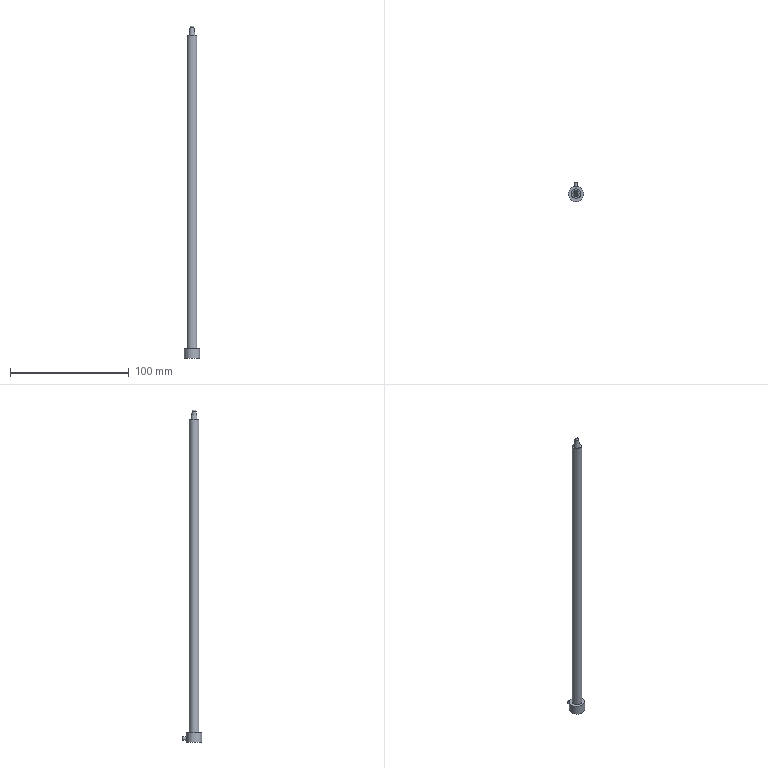Part | STEP file | E108-15-310 | 1 solid | 11 faces | box 13 x 16.5 x 280 mm | volume 14461 mm3 | plane 5 | cylinder 3 | cone 2 | spline 1 | commonest cylinder face diameters 3 x1 8 x1 13 x1
STEP:
#1=CARTESIAN_POINT('',(0.,0.,0.));
#2=DIRECTION('',(0.,0.,1.));
#3=DIRECTION('',(1.,0.,0.));
#4=AXIS2_PLACEMENT_3D('',#1,#2,#3);
#5=CARTESIAN_POINT('',(-4.,0.,272.));
#6=VERTEX_POINT('',#5);
#7=CARTESIAN_POINT('',(4.,0.,272.));
#8=VERTEX_POINT('',#7);
#9=CARTESIAN_POINT('',(0.,0.,272.));
#10=DIRECTION('',(0.,0.,1.));
#11=DIRECTION('',(1.,0.,0.));
#12=AXIS2_PLACEMENT_3D('',#9,#10,#11);
#13=CIRCLE('',#12,4.);
#14=CARTESIAN_POINT('',(0.,0.,100.));
#15=DIRECTION('',(0.,0.,-1.));
#16=DIRECTION('',(-1.,0.,0.));
#17=AXIS2_PLACEMENT_3D('',#14,#15,#16);
#18=CYLINDRICAL_SURFACE('',#17,4.);
#19=CARTESIAN_POINT('',(9.425,-172.));
#20=DIRECTION('',(-1.,0.));
#21=VECTOR('',#20,1.);
#22=LINE('',#19,#21);
#23=(GEOMETRIC_REPRESENTATION_CONTEXT(2)PARAMETRIC_REPRESENTATION_CONTEXT()REPRESENTATION_CONTEXT('',''));
#24=DEFINITIONAL_REPRESENTATION('',(#22),#23);
#25=PCURVE('',#18,#24);
#26=CARTESIAN_POINT('',(0.,0.,272.));
#27=DIRECTION('',(0.,0.,1.));
#28=DIRECTION('',(1.,0.,0.));
#29=AXIS2_PLACEMENT_3D('',#26,#27,#28);
#30=PLANE('',#29);
#31=CARTESIAN_POINT('',(0.,0.));
#32=DIRECTION('',(1.,0.));
#33=AXIS2_PLACEMENT_2D('',#31,#32);
#34=CIRCLE('',#33,4.);
#35=(GEOMETRIC_REPRESENTATION_CONTEXT(2)PARAMETRIC_REPRESENTATION_CONTEXT()REPRESENTATION_CONTEXT('',''));
#36=DEFINITIONAL_REPRESENTATION('',(#34),#35);
#37=PCURVE('',#30,#36);
#38=SURFACE_CURVE('',#13,(#25,#37),.PCURVE_S1.);
#39=EDGE_CURVE('',#6,#8,#38,.T.);
#40=ORIENTED_EDGE('',*,*,#39,.F.);
#41=CARTESIAN_POINT('',(-4.,0.,8.));
#42=VERTEX_POINT('',#41);
#43=CARTESIAN_POINT('',(-4.,0.,272.));
#44=CARTESIAN_POINT('',(-4.,0.,8.));
#45=B_SPLINE_CURVE_WITH_KNOTS('',1,(#43,#44),.UNSPECIFIED.,.F.,.F.,(2,2),(-172.,92.),.PIECEWISE_BEZIER_KNOTS.);
#46=CARTESIAN_POINT('',(6.283,0.));
#47=DIRECTION('',(0.,1.));
#48=VECTOR('',#47,1.);
#49=LINE('',#46,#48);
#50=(GEOMETRIC_REPRESENTATION_CONTEXT(2)PARAMETRIC_REPRESENTATION_CONTEXT()REPRESENTATION_CONTEXT('',''));
#51=DEFINITIONAL_REPRESENTATION('',(#49),#50);
#52=PCURVE('',#18,#51);
#53=CARTESIAN_POINT('',(0.,0.));
#54=DIRECTION('',(0.,1.));
#55=VECTOR('',#54,1.);
#56=LINE('',#53,#55);
#57=(GEOMETRIC_REPRESENTATION_CONTEXT(2)PARAMETRIC_REPRESENTATION_CONTEXT()REPRESENTATION_CONTEXT('',''));
#58=DEFINITIONAL_REPRESENTATION('',(#56),#57);
#59=PCURVE('',#18,#58);
#60=SEAM_CURVE('',#45,(#52,#59),.PCURVE_S1.);
#61=EDGE_CURVE('',#6,#42,#60,.T.);
#62=ORIENTED_EDGE('',*,*,#61,.T.);
#63=CARTESIAN_POINT('',(0.,0.,8.));
#64=DIRECTION('',(0.,0.,1.));
#65=DIRECTION('',(-1.,0.,0.));
#66=AXIS2_PLACEMENT_3D('',#63,#64,#65);
#67=CIRCLE('',#66,4.);
#68=CARTESIAN_POINT('',(6.283,92.));
#69=DIRECTION('',(-1.,0.));
#70=VECTOR('',#69,1.);
#71=LINE('',#68,#70);
#72=(GEOMETRIC_REPRESENTATION_CONTEXT(2)PARAMETRIC_REPRESENTATION_CONTEXT()REPRESENTATION_CONTEXT('',''));
#73=DEFINITIONAL_REPRESENTATION('',(#71),#72);
#74=PCURVE('',#18,#73);
#75=CARTESIAN_POINT('',(0.,0.,8.));
#76=DIRECTION('',(0.,0.,-1.));
#77=DIRECTION('',(1.,0.,0.));
#78=AXIS2_PLACEMENT_3D('',#75,#76,#77);
#79=PLANE('',#78);
#80=CARTESIAN_POINT('',(-4.,0.));
#81=CARTESIAN_POINT('',(-4.,6.928));
#82=CARTESIAN_POINT('',(2.,3.464));
#83=CARTESIAN_POINT('',(8.,0.));
#84=CARTESIAN_POINT('',(2.,-3.464));
#85=CARTESIAN_POINT('',(-4.,-6.928));
#86=CARTESIAN_POINT('',(-4.,0.));
#87=(BOUNDED_CURVE()B_SPLINE_CURVE(2,(#80,#81,#82,#83,#84,#85,#86),.UNSPECIFIED.,.T.,.F.)B_SPLINE_CURVE_WITH_KNOTS((1,2,2,2,2,1),(-2.094,0.,2.094,4.189,6.283,8.378),.UNSPECIFIED.)CURVE()GEOMETRIC_REPRESENTATION_ITEM()RATIONAL_B_SPLINE_CURVE((1.,0.5,1.,0.5,1.,0.5,1.))REPRESENTATION_ITEM(''));
#88=(GEOMETRIC_REPRESENTATION_CONTEXT(2)PARAMETRIC_REPRESENTATION_CONTEXT()REPRESENTATION_CONTEXT('',''));
#89=DEFINITIONAL_REPRESENTATION('',(#87),#88);
#90=PCURVE('',#79,#89);
#91=SURFACE_CURVE('',#67,(#74,#90),.PCURVE_S1.);
#92=EDGE_CURVE('',#42,#42,#91,.T.);
#93=ORIENTED_EDGE('',*,*,#92,.T.);
#94=ORIENTED_EDGE('',*,*,#61,.F.);
#95=CARTESIAN_POINT('',(0.,0.,272.));
#96=DIRECTION('',(0.,0.,1.));
#97=DIRECTION('',(1.,0.,0.));
#98=AXIS2_PLACEMENT_3D('',#95,#96,#97);
#99=CIRCLE('',#98,4.);
#100=CARTESIAN_POINT('',(3.142,-172.));
#101=DIRECTION('',(-1.,0.));
#102=VECTOR('',#101,1.);
#103=LINE('',#100,#102);
#104=(GEOMETRIC_REPRESENTATION_CONTEXT(2)PARAMETRIC_REPRESENTATION_CONTEXT()REPRESENTATION_CONTEXT('',''));
#105=DEFINITIONAL_REPRESENTATION('',(#103),#104);
#106=PCURVE('',#18,#105);
#107=CARTESIAN_POINT('',(0.,0.));
#108=DIRECTION('',(1.,0.));
#109=AXIS2_PLACEMENT_2D('',#107,#108);
#110=CIRCLE('',#109,4.);
#111=(GEOMETRIC_REPRESENTATION_CONTEXT(2)PARAMETRIC_REPRESENTATION_CONTEXT()REPRESENTATION_CONTEXT('',''));
#112=DEFINITIONAL_REPRESENTATION('',(#110),#111);
#113=PCURVE('',#30,#112);
#114=SURFACE_CURVE('',#99,(#106,#113),.PCURVE_S1.);
#115=EDGE_CURVE('',#8,#6,#114,.T.);
#116=ORIENTED_EDGE('',*,*,#115,.F.);
#117=EDGE_LOOP('',(#40,#62,#93,#94,#116));
#118=FACE_BOUND('',#117,.T.);
#119=ADVANCED_FACE('',(#118),#18,.T.);
#120=CARTESIAN_POINT('',(2.553,0.,272.));
#121=VERTEX_POINT('',#120);
#122=CARTESIAN_POINT('',(0.,0.,272.));
#123=DIRECTION('',(0.,0.,1.));
#124=DIRECTION('',(1.,0.,0.));
#125=AXIS2_PLACEMENT_3D('',#122,#123,#124);
#126=CIRCLE('',#125,2.553);
#127=CARTESIAN_POINT('',(0.,0.));
#128=DIRECTION('',(1.,0.));
#129=AXIS2_PLACEMENT_2D('',#127,#128);
#130=CIRCLE('',#129,2.553);
#131=(GEOMETRIC_REPRESENTATION_CONTEXT(2)PARAMETRIC_REPRESENTATION_CONTEXT()REPRESENTATION_CONTEXT('',''));
#132=DEFINITIONAL_REPRESENTATION('',(#130),#131);
#133=PCURVE('',#30,#132);
#134=CARTESIAN_POINT('',(0.,0.,280.));
#135=DIRECTION('',(0.,0.,-1.));
#136=DIRECTION('',(-1.,0.,0.));
#137=AXIS2_PLACEMENT_3D('',#134,#135,#136);
#138=CONICAL_SURFACE('',#137,1.5,0.1309);
#139=CARTESIAN_POINT('',(9.425,8.));
#140=DIRECTION('',(-1.,0.));
#141=VECTOR('',#140,1.);
#142=LINE('',#139,#141);
#143=(GEOMETRIC_REPRESENTATION_CONTEXT(2)PARAMETRIC_REPRESENTATION_CONTEXT()REPRESENTATION_CONTEXT('',''));
#144=DEFINITIONAL_REPRESENTATION('',(#142),#143);
#145=PCURVE('',#138,#144);
#146=SURFACE_CURVE('',#126,(#133,#145),.PCURVE_S1.);
#147=EDGE_CURVE('',#121,#121,#146,.T.);
#148=ORIENTED_EDGE('',*,*,#147,.F.);
#149=EDGE_LOOP('',(#148));
#150=FACE_BOUND('',#149,.T.);
#151=ORIENTED_EDGE('',*,*,#115,.T.);
#152=ORIENTED_EDGE('',*,*,#39,.T.);
#153=EDGE_LOOP('',(#151,#152));
#154=FACE_BOUND('',#153,.T.);
#155=ADVANCED_FACE('',(#150,#154),#30,.T.);
#156=CARTESIAN_POINT('',(6.5,0.,0.));
#157=VERTEX_POINT('',#156);
#158=CARTESIAN_POINT('',(-6.5,0.,0.));
#159=VERTEX_POINT('',#158);
#160=CARTESIAN_POINT('',(0.,0.,0.));
#161=DIRECTION('',(0.,0.,-1.));
#162=DIRECTION('',(-1.,0.,0.));
#163=AXIS2_PLACEMENT_3D('',#160,#161,#162);
#164=CIRCLE('',#163,6.5);
#165=CARTESIAN_POINT('',(0.,0.,8.));
#166=DIRECTION('',(0.,0.,-1.));
#167=DIRECTION('',(1.,0.,0.));
#168=AXIS2_PLACEMENT_3D('',#165,#166,#167);
#169=CYLINDRICAL_SURFACE('',#168,6.5);
#170=CARTESIAN_POINT('',(-3.142,8.));
#171=DIRECTION('',(1.,0.));
#172=VECTOR('',#171,1.);
#173=LINE('',#170,#172);
#174=(GEOMETRIC_REPRESENTATION_CONTEXT(2)PARAMETRIC_REPRESENTATION_CONTEXT()REPRESENTATION_CONTEXT('',''));
#175=DEFINITIONAL_REPRESENTATION('',(#173),#174);
#176=PCURVE('',#169,#175);
#177=CARTESIAN_POINT('',(240.,-1000.,0.));
#178=DIRECTION('',(0.,0.,1.));
#179=DIRECTION('',(-1.,0.,0.));
#180=AXIS2_PLACEMENT_3D('',#177,#178,#179);
#181=PLANE('',#180);
#182=CARTESIAN_POINT('',(246.5,-1000.));
#183=CARTESIAN_POINT('',(246.5,-1011.258));
#184=CARTESIAN_POINT('',(236.75,-1005.629));
#185=CARTESIAN_POINT('',(227.,-1000.));
#186=CARTESIAN_POINT('',(236.75,-994.371));
#187=CARTESIAN_POINT('',(246.5,-988.742));
#188=CARTESIAN_POINT('',(246.5,-1000.));
#189=(BOUNDED_CURVE()B_SPLINE_CURVE(2,(#182,#183,#184,#185,#186,#187,#188),.UNSPECIFIED.,.T.,.F.)B_SPLINE_CURVE_WITH_KNOTS((1,2,2,2,2,1),(-2.094,0.,2.094,4.189,6.283,8.378),.UNSPECIFIED.)CURVE()GEOMETRIC_REPRESENTATION_ITEM()RATIONAL_B_SPLINE_CURVE((1.,0.5,1.,0.5,1.,0.5,1.))REPRESENTATION_ITEM(''));
#190=(GEOMETRIC_REPRESENTATION_CONTEXT(2)PARAMETRIC_REPRESENTATION_CONTEXT()REPRESENTATION_CONTEXT('',''));
#191=DEFINITIONAL_REPRESENTATION('',(#189),#190);
#192=PCURVE('',#181,#191);
#193=SURFACE_CURVE('',#164,(#176,#192),.PCURVE_S1.);
#194=EDGE_CURVE('',#157,#159,#193,.T.);
#195=ORIENTED_EDGE('',*,*,#194,.F.);
#196=CARTESIAN_POINT('',(6.5,0.,8.));
#197=VERTEX_POINT('',#196);
#198=CARTESIAN_POINT('',(6.5,0.,8.));
#199=CARTESIAN_POINT('',(6.5,0.,0.));
#200=B_SPLINE_CURVE_WITH_KNOTS('',1,(#198,#199),.UNSPECIFIED.,.F.,.F.,(2,2),(0.,8.),.PIECEWISE_BEZIER_KNOTS.);
#201=CARTESIAN_POINT('',(0.,0.));
#202=DIRECTION('',(0.,1.));
#203=VECTOR('',#202,1.);
#204=LINE('',#201,#203);
#205=(GEOMETRIC_REPRESENTATION_CONTEXT(2)PARAMETRIC_REPRESENTATION_CONTEXT()REPRESENTATION_CONTEXT('',''));
#206=DEFINITIONAL_REPRESENTATION('',(#204),#205);
#207=PCURVE('',#169,#206);
#208=CARTESIAN_POINT('',(6.283,0.));
#209=DIRECTION('',(0.,1.));
#210=VECTOR('',#209,1.);
#211=LINE('',#208,#210);
#212=(GEOMETRIC_REPRESENTATION_CONTEXT(2)PARAMETRIC_REPRESENTATION_CONTEXT()REPRESENTATION_CONTEXT('',''));
#213=DEFINITIONAL_REPRESENTATION('',(#211),#212);
#214=PCURVE('',#169,#213);
#215=SEAM_CURVE('',#200,(#207,#214),.PCURVE_S1.);
#216=EDGE_CURVE('',#197,#157,#215,.T.);
#217=ORIENTED_EDGE('',*,*,#216,.F.);
#218=CARTESIAN_POINT('',(0.,0.,8.));
#219=DIRECTION('',(0.,0.,-1.));
#220=DIRECTION('',(1.,0.,0.));
#221=AXIS2_PLACEMENT_3D('',#218,#219,#220);
#222=CIRCLE('',#221,6.5);
#223=CARTESIAN_POINT('',(0.,0.));
#224=DIRECTION('',(1.,0.));
#225=VECTOR('',#224,1.);
#226=LINE('',#223,#225);
#227=(GEOMETRIC_REPRESENTATION_CONTEXT(2)PARAMETRIC_REPRESENTATION_CONTEXT()REPRESENTATION_CONTEXT('',''));
#228=DEFINITIONAL_REPRESENTATION('',(#226),#227);
#229=PCURVE('',#169,#228);
#230=CARTESIAN_POINT('',(0.,0.));
#231=DIRECTION('',(1.,0.));
#232=AXIS2_PLACEMENT_2D('',#230,#231);
#233=CIRCLE('',#232,6.5);
#234=(GEOMETRIC_REPRESENTATION_CONTEXT(2)PARAMETRIC_REPRESENTATION_CONTEXT()REPRESENTATION_CONTEXT('',''));
#235=DEFINITIONAL_REPRESENTATION('',(#233),#234);
#236=PCURVE('',#79,#235);
#237=SURFACE_CURVE('',#222,(#229,#236),.PCURVE_S1.);
#238=EDGE_CURVE('',#197,#197,#237,.T.);
#239=ORIENTED_EDGE('',*,*,#238,.T.);
#240=ORIENTED_EDGE('',*,*,#216,.T.);
#241=CARTESIAN_POINT('',(0.,0.,0.));
#242=DIRECTION('',(0.,0.,-1.));
#243=DIRECTION('',(-1.,0.,0.));
#244=AXIS2_PLACEMENT_3D('',#241,#242,#243);
#245=CIRCLE('',#244,6.5);
#246=CARTESIAN_POINT('',(3.142,8.));
#247=DIRECTION('',(1.,0.));
#248=VECTOR('',#247,1.);
#249=LINE('',#246,#248);
#250=(GEOMETRIC_REPRESENTATION_CONTEXT(2)PARAMETRIC_REPRESENTATION_CONTEXT()REPRESENTATION_CONTEXT('',''));
#251=DEFINITIONAL_REPRESENTATION('',(#249),#250);
#252=PCURVE('',#169,#251);
#253=CARTESIAN_POINT('',(246.5,-1000.));
#254=CARTESIAN_POINT('',(246.5,-1011.258));
#255=CARTESIAN_POINT('',(236.75,-1005.629));
#256=CARTESIAN_POINT('',(227.,-1000.));
#257=CARTESIAN_POINT('',(236.75,-994.371));
#258=CARTESIAN_POINT('',(246.5,-988.742));
#259=CARTESIAN_POINT('',(246.5,-1000.));
#260=(BOUNDED_CURVE()B_SPLINE_CURVE(2,(#253,#254,#255,#256,#257,#258,#259),.UNSPECIFIED.,.T.,.F.)B_SPLINE_CURVE_WITH_KNOTS((1,2,2,2,2,1),(-2.094,0.,2.094,4.189,6.283,8.378),.UNSPECIFIED.)CURVE()GEOMETRIC_REPRESENTATION_ITEM()RATIONAL_B_SPLINE_CURVE((1.,0.5,1.,0.5,1.,0.5,1.))REPRESENTATION_ITEM(''));
#261=(GEOMETRIC_REPRESENTATION_CONTEXT(2)PARAMETRIC_REPRESENTATION_CONTEXT()REPRESENTATION_CONTEXT('',''));
#262=DEFINITIONAL_REPRESENTATION('',(#260),#261);
#263=PCURVE('',#181,#262);
#264=SURFACE_CURVE('',#245,(#252,#263),.PCURVE_S1.);
#265=EDGE_CURVE('',#159,#157,#264,.T.);
#266=ORIENTED_EDGE('',*,*,#265,.F.);
#267=EDGE_LOOP('',(#195,#217,#239,#240,#266));
#268=FACE_BOUND('',#267,.T.);
#269=CARTESIAN_POINT('',(0.,6.5,1.5));
#270=VERTEX_POINT('',#269);
#271=CARTESIAN_POINT('',(0.,6.5,1.5));
#272=CARTESIAN_POINT('',(0.1654,6.5,1.5));
#273=CARTESIAN_POINT('',(0.3332,6.493,1.528));
#274=CARTESIAN_POINT('',(0.4892,6.482,1.582));
#275=CARTESIAN_POINT('',(0.6451,6.47,1.636));
#276=CARTESIAN_POINT('',(0.7936,6.453,1.717));
#277=CARTESIAN_POINT('',(0.9231,6.434,1.818));
#278=CARTESIAN_POINT('',(1.055,6.415,1.92));
#279=CARTESIAN_POINT('',(1.17,6.394,2.047));
#280=CARTESIAN_POINT('',(1.261,6.377,2.187));
#281=CARTESIAN_POINT('',(1.352,6.358,2.329));
#282=CARTESIAN_POINT('',(1.421,6.343,2.49));
#283=CARTESIAN_POINT('',(1.46,6.334,2.655));
#284=CARTESIAN_POINT('',(1.498,6.325,2.817));
#285=CARTESIAN_POINT('',(1.509,6.322,2.989));
#286=CARTESIAN_POINT('',(1.492,6.326,3.155));
#287=CARTESIAN_POINT('',(1.475,6.33,3.318));
#288=CARTESIAN_POINT('',(1.431,6.341,3.48));
#289=CARTESIAN_POINT('',(1.362,6.356,3.628));
#290=CARTESIAN_POINT('',(1.293,6.37,3.777));
#291=CARTESIAN_POINT('',(1.199,6.39,3.917));
#292=CARTESIAN_POINT('',(1.085,6.409,4.035));
#293=CARTESIAN_POINT('',(0.9695,6.428,4.157));
#294=CARTESIAN_POINT('',(0.8309,6.448,4.26));
#295=CARTESIAN_POINT('',(0.6809,6.464,4.337));
#296=CARTESIAN_POINT('',(0.5305,6.48,4.413));
#297=CARTESIAN_POINT('',(0.3642,6.492,4.465));
#298=CARTESIAN_POINT('',(0.1962,6.497,4.487));
#299=CARTESIAN_POINT('',(0.03191,6.502,4.509));
#300=CARTESIAN_POINT('',(-0.1386,6.501,4.503));
#301=CARTESIAN_POINT('',(-0.3008,6.493,4.47));
#302=CARTESIAN_POINT('',(-0.4611,6.486,4.437));
#303=CARTESIAN_POINT('',(-0.6177,6.472,4.377));
#304=CARTESIAN_POINT('',(-0.7583,6.456,4.294));
#305=CARTESIAN_POINT('',(-0.9011,6.439,4.211));
#306=CARTESIAN_POINT('',(-1.031,6.419,4.102));
#307=CARTESIAN_POINT('',(-1.139,6.399,3.976));
#308=CARTESIAN_POINT('',(-1.249,6.38,3.848));
#309=CARTESIAN_POINT('',(-1.338,6.361,3.699));
#310=CARTESIAN_POINT('',(-1.399,6.348,3.541));
#311=CARTESIAN_POINT('',(-1.46,6.334,3.384));
#312=CARTESIAN_POINT('',(-1.494,6.326,3.214));
#313=CARTESIAN_POINT('',(-1.499,6.325,3.046));
#314=CARTESIAN_POINT('',(-1.504,6.324,2.881));
#315=CARTESIAN_POINT('',(-1.482,6.329,2.714));
#316=CARTESIAN_POINT('',(-1.433,6.34,2.557));
#317=CARTESIAN_POINT('',(-1.385,6.351,2.4));
#318=CARTESIAN_POINT('',(-1.309,6.367,2.25));
#319=CARTESIAN_POINT('',(-1.214,6.386,2.119));
#320=CARTESIAN_POINT('',(-1.116,6.404,1.984));
#321=CARTESIAN_POINT('',(-0.9937,6.425,1.864));
#322=CARTESIAN_POINT('',(-0.8569,6.443,1.769));
#323=CARTESIAN_POINT('',(-0.7182,6.462,1.672));
#324=CARTESIAN_POINT('',(-0.5604,6.478,1.598));
#325=CARTESIAN_POINT('',(-0.3967,6.488,1.553));
#326=CARTESIAN_POINT('',(-0.2682,6.496,1.518));
#327=CARTESIAN_POINT('',(-0.1335,6.5,1.5));
#328=CARTESIAN_POINT('',(0.,6.5,1.5));
#329=B_SPLINE_CURVE_WITH_KNOTS('',3,(#271,#272,#273,#274,#275,#276,#277,#278,#279,#280,#281,#282,#283,#284,#285,#286,#287,#288,#289,#290,#291,#292,#293,#294,#295,#296,#297,#298,#299,#300,#301,#302,#303,#304,#305,#306,#307,#308,#309,#310,#311,#312,#313,#314,#315,#316,#317,#318,#319,#320,#321,#322,#323,#324,#325,#326,#327,#328),.UNSPECIFIED.,.T.,.F.,(1,3,3,3,3,3,3,3,3,3,3,3,3,3,3,3,3,3,3,3,3,1),(-0.04234,0.,0.05275,0.1054,0.159,0.2132,0.2665,0.3187,0.3713,0.4252,0.4793,0.5321,0.5843,0.6373,0.6915,0.7453,0.7978,0.85,0.9034,0.9577,1.,1.053),.UNSPECIFIED.);
#330=CARTESIAN_POINT('',(4.712,6.5));
#331=CARTESIAN_POINT('',(4.718,6.5));
#332=CARTESIAN_POINT('',(4.729,6.497));
#333=CARTESIAN_POINT('',(4.745,6.486));
#334=CARTESIAN_POINT('',(4.762,6.467));
#335=CARTESIAN_POINT('',(4.778,6.44));
#336=CARTESIAN_POINT('',(4.793,6.406));
#337=CARTESIAN_POINT('',(4.809,6.365));
#338=CARTESIAN_POINT('',(4.823,6.317));
#339=CARTESIAN_POINT('',(4.838,6.262));
#340=CARTESIAN_POINT('',(4.851,6.201));
#341=CARTESIAN_POINT('',(4.864,6.135));
#342=CARTESIAN_POINT('',(4.876,6.062));
#343=CARTESIAN_POINT('',(4.888,5.983));
#344=CARTESIAN_POINT('',(4.898,5.9));
#345=CARTESIAN_POINT('',(4.908,5.813));
#346=CARTESIAN_POINT('',(4.916,5.721));
#347=CARTESIAN_POINT('',(4.924,5.625));
#348=CARTESIAN_POINT('',(4.93,5.526));
#349=CARTESIAN_POINT('',(4.936,5.424));
#350=CARTESIAN_POINT('',(4.94,5.321));
#351=CARTESIAN_POINT('',(4.943,5.215));
#352=CARTESIAN_POINT('',(4.945,5.108));
#353=CARTESIAN_POINT('',(4.945,5.));
#354=CARTESIAN_POINT('',(4.945,4.893));
#355=CARTESIAN_POINT('',(4.943,4.787));
#356=CARTESIAN_POINT('',(4.94,4.681));
#357=CARTESIAN_POINT('',(4.936,4.576));
#358=CARTESIAN_POINT('',(4.93,4.474));
#359=CARTESIAN_POINT('',(4.924,4.376));
#360=CARTESIAN_POINT('',(4.916,4.28));
#361=CARTESIAN_POINT('',(4.908,4.188));
#362=CARTESIAN_POINT('',(4.898,4.1));
#363=CARTESIAN_POINT('',(4.888,4.017));
#364=CARTESIAN_POINT('',(4.877,3.939));
#365=CARTESIAN_POINT('',(4.864,3.866));
#366=CARTESIAN_POINT('',(4.851,3.799));
#367=CARTESIAN_POINT('',(4.838,3.738));
#368=CARTESIAN_POINT('',(4.824,3.683));
#369=CARTESIAN_POINT('',(4.809,3.635));
#370=CARTESIAN_POINT('',(4.793,3.594));
#371=CARTESIAN_POINT('',(4.778,3.56));
#372=CARTESIAN_POINT('',(4.762,3.533));
#373=CARTESIAN_POINT('',(4.745,3.514));
#374=CARTESIAN_POINT('',(4.729,3.503));
#375=CARTESIAN_POINT('',(4.713,3.499));
#376=CARTESIAN_POINT('',(4.696,3.503));
#377=CARTESIAN_POINT('',(4.679,3.514));
#378=CARTESIAN_POINT('',(4.663,3.533));
#379=CARTESIAN_POINT('',(4.647,3.56));
#380=CARTESIAN_POINT('',(4.632,3.594));
#381=CARTESIAN_POINT('',(4.616,3.635));
#382=CARTESIAN_POINT('',(4.601,3.683));
#383=CARTESIAN_POINT('',(4.587,3.737));
#384=CARTESIAN_POINT('',(4.574,3.798));
#385=CARTESIAN_POINT('',(4.561,3.865));
#386=CARTESIAN_POINT('',(4.548,3.938));
#387=CARTESIAN_POINT('',(4.537,4.016));
#388=CARTESIAN_POINT('',(4.527,4.099));
#389=CARTESIAN_POINT('',(4.517,4.187));
#390=CARTESIAN_POINT('',(4.508,4.279));
#391=CARTESIAN_POINT('',(4.501,4.375));
#392=CARTESIAN_POINT('',(4.494,4.473));
#393=CARTESIAN_POINT('',(4.489,4.575));
#394=CARTESIAN_POINT('',(4.485,4.679));
#395=CARTESIAN_POINT('',(4.482,4.785));
#396=CARTESIAN_POINT('',(4.48,4.892));
#397=CARTESIAN_POINT('',(4.479,4.999));
#398=CARTESIAN_POINT('',(4.48,5.106));
#399=CARTESIAN_POINT('',(4.482,5.213));
#400=CARTESIAN_POINT('',(4.485,5.319));
#401=CARTESIAN_POINT('',(4.489,5.423));
#402=CARTESIAN_POINT('',(4.494,5.524));
#403=CARTESIAN_POINT('',(4.501,5.624));
#404=CARTESIAN_POINT('',(4.508,5.72));
#405=CARTESIAN_POINT('',(4.517,5.812));
#406=CARTESIAN_POINT('',(4.526,5.899));
#407=CARTESIAN_POINT('',(4.537,5.982));
#408=CARTESIAN_POINT('',(4.548,6.061));
#409=CARTESIAN_POINT('',(4.56,6.134));
#410=CARTESIAN_POINT('',(4.573,6.201));
#411=CARTESIAN_POINT('',(4.587,6.262));
#412=CARTESIAN_POINT('',(4.601,6.316));
#413=CARTESIAN_POINT('',(4.616,6.364));
#414=CARTESIAN_POINT('',(4.631,6.406));
#415=CARTESIAN_POINT('',(4.647,6.44));
#416=CARTESIAN_POINT('',(4.663,6.466));
#417=CARTESIAN_POINT('',(4.679,6.486));
#418=CARTESIAN_POINT('',(4.696,6.497));
#419=CARTESIAN_POINT('',(4.707,6.5));
#420=CARTESIAN_POINT('',(4.712,6.5));
#421=B_SPLINE_CURVE_WITH_KNOTS('',3,(#330,#331,#332,#333,#334,#335,#336,#337,#338,#339,#340,#341,#342,#343,#344,#345,#346,#347,#348,#349,#350,#351,#352,#353,#354,#355,#356,#357,#358,#359,#360,#361,#362,#363,#364,#365,#366,#367,#368,#369,#370,#371,#372,#373,#374,#375,#376,#377,#378,#379,#380,#381,#382,#383,#384,#385,#386,#387,#388,#389,#390,#391,#392,#393,#394,#395,#396,#397,#398,#399,#400,#401,#402,#403,#404,#405,#406,#407,#408,#409,#410,#411,#412,#413,#414,#415,#416,#417,#418,#419,#420),.UNSPECIFIED.,.T.,.F.,(4,1,1,1,1,1,1,1,1,1,1,1,1,1,1,1,1,1,1,1,1,1,1,1,1,1,1,1,1,1,1,1,1,1,1,1,1,1,1,1,1,1,1,1,1,1,1,1,1,1,1,1,1,1,1,1,1,1,1,1,1,1,1,1,1,1,1,1,1,1,1,1,1,1,1,1,1,1,1,1,1,1,1,1,1,1,1,1,4),(0.,0.01136,0.02273,0.03409,0.04545,0.05682,0.06818,0.07955,0.09091,0.1023,0.1136,0.125,0.1364,0.1477,0.1591,0.1705,0.1818,0.1932,0.2045,0.2159,0.2273,0.2386,0.25,0.2614,0.2727,0.2841,0.2955,0.3068,0.3182,0.3295,0.3409,0.3523,0.3636,0.375,0.3864,0.3977,0.4091,0.4205,0.4318,0.4432,0.4545,0.4659,0.4773,0.4886,0.5,0.5114,0.5227,0.5341,0.5455,0.5568,0.5682,0.5795,0.5909,0.6023,0.6136,0.625,0.6364,0.6477,0.6591,0.6705,0.6818,0.6932,0.7045,0.7159,0.7273,0.7386,0.75,0.7614,0.7727,0.7841,0.7955,0.8068,0.8182,0.8295,0.8409,0.8523,0.8636,0.875,0.8864,0.8977,0.9091,0.9205,0.9318,0.9432,0.9545,0.9659,0.9773,0.9886,1.),.QUASI_UNIFORM_KNOTS.);
#422=(GEOMETRIC_REPRESENTATION_CONTEXT(2)PARAMETRIC_REPRESENTATION_CONTEXT()REPRESENTATION_CONTEXT('',''));
#423=DEFINITIONAL_REPRESENTATION('',(#421),#422);
#424=PCURVE('',#169,#423);
#425=CARTESIAN_POINT('',(0.,2.,3.));
#426=DIRECTION('',(0.,1.,0.));
#427=DIRECTION('',(0.,0.,-1.));
#428=AXIS2_PLACEMENT_3D('',#425,#426,#427);
#429=CYLINDRICAL_SURFACE('',#428,1.5);
#430=CARTESIAN_POINT('',(6.283,4.5));
#431=CARTESIAN_POINT('',(6.259,4.5));
#432=CARTESIAN_POINT('',(6.212,4.499));
#433=CARTESIAN_POINT('',(6.14,4.497));
#434=CARTESIAN_POINT('',(6.068,4.492));
#435=CARTESIAN_POINT('',(5.997,4.486));
#436=CARTESIAN_POINT('',(5.926,4.479));
#437=CARTESIAN_POINT('',(5.854,4.47));
#438=CARTESIAN_POINT('',(5.783,4.46));
#439=CARTESIAN_POINT('',(5.711,4.449));
#440=CARTESIAN_POINT('',(5.64,4.438));
#441=CARTESIAN_POINT('',(5.569,4.425));
#442=CARTESIAN_POINT('',(5.498,4.413));
#443=CARTESIAN_POINT('',(5.427,4.4));
#444=CARTESIAN_POINT('',(5.355,4.388));
#445=CARTESIAN_POINT('',(5.284,4.376));
#446=CARTESIAN_POINT('',(5.213,4.365));
#447=CARTESIAN_POINT('',(5.142,4.355));
#448=CARTESIAN_POINT('',(5.07,4.346));
#449=CARTESIAN_POINT('',(4.999,4.338));
#450=CARTESIAN_POINT('',(4.928,4.332));
#451=CARTESIAN_POINT('',(4.856,4.328));
#452=CARTESIAN_POINT('',(4.784,4.325));
#453=CARTESIAN_POINT('',(4.713,4.324));
#454=CARTESIAN_POINT('',(4.641,4.325));
#455=CARTESIAN_POINT('',(4.57,4.328));
#456=CARTESIAN_POINT('',(4.498,4.332));
#457=CARTESIAN_POINT('',(4.426,4.339));
#458=CARTESIAN_POINT('',(4.355,4.346));
#459=CARTESIAN_POINT('',(4.283,4.355));
#460=CARTESIAN_POINT('',(4.212,4.365));
#461=CARTESIAN_POINT('',(4.141,4.376));
#462=CARTESIAN_POINT('',(4.07,4.388));
#463=CARTESIAN_POINT('',(3.998,4.4));
#464=CARTESIAN_POINT('',(3.927,4.413));
#465=CARTESIAN_POINT('',(3.856,4.425));
#466=CARTESIAN_POINT('',(3.785,4.437));
#467=CARTESIAN_POINT('',(3.714,4.449));
#468=CARTESIAN_POINT('',(3.642,4.46));
#469=CARTESIAN_POINT('',(3.571,4.47));
#470=CARTESIAN_POINT('',(3.5,4.479));
#471=CARTESIAN_POINT('',(3.428,4.486));
#472=CARTESIAN_POINT('',(3.357,4.492));
#473=CARTESIAN_POINT('',(3.285,4.497));
#474=CARTESIAN_POINT('',(3.214,4.499));
#475=CARTESIAN_POINT('',(3.142,4.5));
#476=CARTESIAN_POINT('',(3.07,4.499));
#477=CARTESIAN_POINT('',(2.999,4.497));
#478=CARTESIAN_POINT('',(2.927,4.492));
#479=CARTESIAN_POINT('',(2.856,4.486));
#480=CARTESIAN_POINT('',(2.784,4.479));
#481=CARTESIAN_POINT('',(2.713,4.47));
#482=CARTESIAN_POINT('',(2.641,4.46));
#483=CARTESIAN_POINT('',(2.57,4.449));
#484=CARTESIAN_POINT('',(2.499,4.438));
#485=CARTESIAN_POINT('',(2.428,4.425));
#486=CARTESIAN_POINT('',(2.357,4.413));
#487=CARTESIAN_POINT('',(2.285,4.4));
#488=CARTESIAN_POINT('',(2.215,4.388));
#489=CARTESIAN_POINT('',(2.143,4.376));
#490=CARTESIAN_POINT('',(2.072,4.365));
#491=CARTESIAN_POINT('',(2.,4.355));
#492=CARTESIAN_POINT('',(1.929,4.346));
#493=CARTESIAN_POINT('',(1.858,4.339));
#494=CARTESIAN_POINT('',(1.786,4.332));
#495=CARTESIAN_POINT('',(1.715,4.328));
#496=CARTESIAN_POINT('',(1.643,4.325));
#497=CARTESIAN_POINT('',(1.572,4.324));
#498=CARTESIAN_POINT('',(1.5,4.325));
#499=CARTESIAN_POINT('',(1.428,4.328));
#500=CARTESIAN_POINT('',(1.357,4.332));
#501=CARTESIAN_POINT('',(1.285,4.338));
#502=CARTESIAN_POINT('',(1.214,4.346));
#503=CARTESIAN_POINT('',(1.142,4.355));
#504=CARTESIAN_POINT('',(1.071,4.365));
#505=CARTESIAN_POINT('',(0.9995,4.376));
#506=CARTESIAN_POINT('',(0.9286,4.388));
#507=CARTESIAN_POINT('',(0.8575,4.4));
#508=CARTESIAN_POINT('',(0.7862,4.413));
#509=CARTESIAN_POINT('',(0.7149,4.425));
#510=CARTESIAN_POINT('',(0.6436,4.437));
#511=CARTESIAN_POINT('',(0.5728,4.449));
#512=CARTESIAN_POINT('',(0.5015,4.46));
#513=CARTESIAN_POINT('',(0.43,4.47));
#514=CARTESIAN_POINT('',(0.3585,4.479));
#515=CARTESIAN_POINT('',(0.2872,4.486));
#516=CARTESIAN_POINT('',(0.2157,4.492));
#517=CARTESIAN_POINT('',(0.1438,4.497));
#518=CARTESIAN_POINT('',(0.07178,4.499));
#519=CARTESIAN_POINT('',(0.02388,4.5));
#520=CARTESIAN_POINT('',(0.,4.5));
#521=B_SPLINE_CURVE_WITH_KNOTS('',3,(#430,#431,#432,#433,#434,#435,#436,#437,#438,#439,#440,#441,#442,#443,#444,#445,#446,#447,#448,#449,#450,#451,#452,#453,#454,#455,#456,#457,#458,#459,#460,#461,#462,#463,#464,#465,#466,#467,#468,#469,#470,#471,#472,#473,#474,#475,#476,#477,#478,#479,#480,#481,#482,#483,#484,#485,#486,#487,#488,#489,#490,#491,#492,#493,#494,#495,#496,#497,#498,#499,#500,#501,#502,#503,#504,#505,#506,#507,#508,#509,#510,#511,#512,#513,#514,#515,#516,#517,#518,#519,#520),.UNSPECIFIED.,.F.,.F.,(4,1,1,1,1,1,1,1,1,1,1,1,1,1,1,1,1,1,1,1,1,1,1,1,1,1,1,1,1,1,1,1,1,1,1,1,1,1,1,1,1,1,1,1,1,1,1,1,1,1,1,1,1,1,1,1,1,1,1,1,1,1,1,1,1,1,1,1,1,1,1,1,1,1,1,1,1,1,1,1,1,1,1,1,1,1,1,1,4),(0.,0.01136,0.02273,0.03409,0.04545,0.05682,0.06818,0.07955,0.09091,0.1023,0.1136,0.125,0.1364,0.1477,0.1591,0.1705,0.1818,0.1932,0.2045,0.2159,0.2273,0.2386,0.25,0.2614,0.2727,0.2841,0.2955,0.3068,0.3182,0.3295,0.3409,0.3523,0.3636,0.375,0.3864,0.3977,0.4091,0.4205,0.4318,0.4432,0.4545,0.4659,0.4773,0.4886,0.5,0.5114,0.5227,0.5341,0.5455,0.5568,0.5682,0.5795,0.5909,0.6023,0.6136,0.625,0.6364,0.6477,0.6591,0.6705,0.6818,0.6932,0.7045,0.7159,0.7273,0.7386,0.75,0.7614,0.7727,0.7841,0.7955,0.8068,0.8182,0.8295,0.8409,0.8523,0.8636,0.875,0.8864,0.8977,0.9091,0.9205,0.9318,0.9432,0.9545,0.9659,0.9773,0.9886,1.),.QUASI_UNIFORM_KNOTS.);
#522=(GEOMETRIC_REPRESENTATION_CONTEXT(2)PARAMETRIC_REPRESENTATION_CONTEXT()REPRESENTATION_CONTEXT('',''));
#523=DEFINITIONAL_REPRESENTATION('',(#521),#522);
#524=PCURVE('',#429,#523);
#525=SURFACE_CURVE('',#329,(#424,#524),.PCURVE_S1.);
#526=EDGE_CURVE('',#270,#270,#525,.T.);
#527=ORIENTED_EDGE('',*,*,#526,.T.);
#528=EDGE_LOOP('',(#527));
#529=FACE_BOUND('',#528,.T.);
#530=ADVANCED_FACE('',(#268,#529),#169,.T.);
#531=ORIENTED_EDGE('',*,*,#92,.F.);
#532=EDGE_LOOP('',(#531));
#533=FACE_BOUND('',#532,.T.);
#534=ORIENTED_EDGE('',*,*,#238,.F.);
#535=EDGE_LOOP('',(#534));
#536=FACE_BOUND('',#535,.T.);
#537=ADVANCED_FACE('',(#533,#536),#79,.F.);
#538=ORIENTED_EDGE('',*,*,#265,.T.);
#539=ORIENTED_EDGE('',*,*,#194,.T.);
#540=EDGE_LOOP('',(#538,#539));
#541=FACE_BOUND('',#540,.T.);
#542=ADVANCED_FACE('',(#541),#181,.F.);
#543=CARTESIAN_POINT('',(0.,10.,1.75));
#544=VERTEX_POINT('',#543);
#545=CARTESIAN_POINT('',(0.,10.,3.));
#546=DIRECTION('',(0.,1.,0.));
#547=DIRECTION('',(0.,0.,-1.));
#548=AXIS2_PLACEMENT_3D('',#545,#546,#547);
#549=CIRCLE('',#548,1.25);
#550=CARTESIAN_POINT('',(0.,10.,3.));
#551=DIRECTION('',(0.,1.,0.));
#552=DIRECTION('',(0.,0.,-1.));
#553=AXIS2_PLACEMENT_3D('',#550,#551,#552);
#554=PLANE('',#553);
#555=CARTESIAN_POINT('',(0.,0.));
#556=DIRECTION('',(1.,0.));
#557=AXIS2_PLACEMENT_2D('',#555,#556);
#558=CIRCLE('',#557,1.25);
#559=(GEOMETRIC_REPRESENTATION_CONTEXT(2)PARAMETRIC_REPRESENTATION_CONTEXT()REPRESENTATION_CONTEXT('',''));
#560=DEFINITIONAL_REPRESENTATION('',(#558),#559);
#561=PCURVE('',#554,#560);
#562=CARTESIAN_POINT('',(0.,9.75,3.));
#563=DIRECTION('',(0.,-1.,0.));
#564=DIRECTION('',(0.,0.,1.));
#565=AXIS2_PLACEMENT_3D('',#562,#563,#564);
#566=CONICAL_SURFACE('',#565,1.5,0.7854);
#567=CARTESIAN_POINT('',(9.425,-0.25));
#568=DIRECTION('',(-1.,0.));
#569=VECTOR('',#568,1.);
#570=LINE('',#567,#569);
#571=(GEOMETRIC_REPRESENTATION_CONTEXT(2)PARAMETRIC_REPRESENTATION_CONTEXT()REPRESENTATION_CONTEXT('',''));
#572=DEFINITIONAL_REPRESENTATION('',(#570),#571);
#573=PCURVE('',#566,#572);
#574=SURFACE_CURVE('',#549,(#561,#573),.PCURVE_S1.);
#575=EDGE_CURVE('',#544,#544,#574,.T.);
#576=ORIENTED_EDGE('',*,*,#575,.T.);
#577=EDGE_LOOP('',(#576));
#578=FACE_BOUND('',#577,.T.);
#579=ADVANCED_FACE('',(#578),#554,.T.);
#580=ORIENTED_EDGE('',*,*,#575,.F.);
#581=CARTESIAN_POINT('',(0.,9.75,1.5));
#582=VERTEX_POINT('',#581);
#583=CARTESIAN_POINT('',(0.,10.,1.75));
#584=CARTESIAN_POINT('',(0.,9.75,1.5));
#585=B_SPLINE_CURVE_WITH_KNOTS('',1,(#583,#584),.UNSPECIFIED.,.F.,.F.,(2,2),(-0.3536,0.),.PIECEWISE_BEZIER_KNOTS.);
#586=CARTESIAN_POINT('',(9.425,0.));
#587=DIRECTION('',(0.,1.));
#588=VECTOR('',#587,1.);
#589=LINE('',#586,#588);
#590=(GEOMETRIC_REPRESENTATION_CONTEXT(2)PARAMETRIC_REPRESENTATION_CONTEXT()REPRESENTATION_CONTEXT('',''));
#591=DEFINITIONAL_REPRESENTATION('',(#589),#590);
#592=PCURVE('',#566,#591);
#593=CARTESIAN_POINT('',(3.142,0.));
#594=DIRECTION('',(0.,1.));
#595=VECTOR('',#594,1.);
#596=LINE('',#593,#595);
#597=(GEOMETRIC_REPRESENTATION_CONTEXT(2)PARAMETRIC_REPRESENTATION_CONTEXT()REPRESENTATION_CONTEXT('',''));
#598=DEFINITIONAL_REPRESENTATION('',(#596),#597);
#599=PCURVE('',#566,#598);
#600=SEAM_CURVE('',#585,(#592,#599),.PCURVE_S1.);
#601=EDGE_CURVE('',#544,#582,#600,.T.);
#602=ORIENTED_EDGE('',*,*,#601,.T.);
#603=CARTESIAN_POINT('',(0.,9.75,3.));
#604=DIRECTION('',(0.,-1.,0.));
#605=DIRECTION('',(0.,0.,-1.));
#606=AXIS2_PLACEMENT_3D('',#603,#604,#605);
#607=CIRCLE('',#606,1.5);
#608=CARTESIAN_POINT('',(3.142,0.));
#609=DIRECTION('',(1.,0.));
#610=VECTOR('',#609,1.);
#611=LINE('',#608,#610);
#612=(GEOMETRIC_REPRESENTATION_CONTEXT(2)PARAMETRIC_REPRESENTATION_CONTEXT()REPRESENTATION_CONTEXT('',''));
#613=DEFINITIONAL_REPRESENTATION('',(#611),#612);
#614=PCURVE('',#566,#613);
#615=CARTESIAN_POINT('',(6.283,7.75));
#616=DIRECTION('',(-1.,0.));
#617=VECTOR('',#616,1.);
#618=LINE('',#615,#617);
#619=(GEOMETRIC_REPRESENTATION_CONTEXT(2)PARAMETRIC_REPRESENTATION_CONTEXT()REPRESENTATION_CONTEXT('',''));
#620=DEFINITIONAL_REPRESENTATION('',(#618),#619);
#621=PCURVE('',#429,#620);
#622=SURFACE_CURVE('',#607,(#614,#621),.PCURVE_S1.);
#623=EDGE_CURVE('',#582,#582,#622,.T.);
#624=ORIENTED_EDGE('',*,*,#623,.F.);
#625=ORIENTED_EDGE('',*,*,#601,.F.);
#626=EDGE_LOOP('',(#580,#602,#624,#625));
#627=FACE_BOUND('',#626,.T.);
#628=ADVANCED_FACE('',(#627),#566,.T.);
#629=ORIENTED_EDGE('',*,*,#526,.F.);
#630=CARTESIAN_POINT('',(0.,6.5,1.5));
#631=CARTESIAN_POINT('',(0.,9.75,1.5));
#632=B_SPLINE_CURVE_WITH_KNOTS('',1,(#630,#631),.UNSPECIFIED.,.F.,.F.,(2,2),(4.5,7.75),.PIECEWISE_BEZIER_KNOTS.);
#633=CARTESIAN_POINT('',(6.283,0.));
#634=DIRECTION('',(0.,1.));
#635=VECTOR('',#634,1.);
#636=LINE('',#633,#635);
#637=(GEOMETRIC_REPRESENTATION_CONTEXT(2)PARAMETRIC_REPRESENTATION_CONTEXT()REPRESENTATION_CONTEXT('',''));
#638=DEFINITIONAL_REPRESENTATION('',(#636),#637);
#639=PCURVE('',#429,#638);
#640=CARTESIAN_POINT('',(0.,0.));
#641=DIRECTION('',(0.,1.));
#642=VECTOR('',#641,1.);
#643=LINE('',#640,#642);
#644=(GEOMETRIC_REPRESENTATION_CONTEXT(2)PARAMETRIC_REPRESENTATION_CONTEXT()REPRESENTATION_CONTEXT('',''));
#645=DEFINITIONAL_REPRESENTATION('',(#643),#644);
#646=PCURVE('',#429,#645);
#647=SEAM_CURVE('',#632,(#639,#646),.PCURVE_S1.);
#648=EDGE_CURVE('',#270,#582,#647,.T.);
#649=ORIENTED_EDGE('',*,*,#648,.T.);
#650=ORIENTED_EDGE('',*,*,#623,.T.);
#651=ORIENTED_EDGE('',*,*,#648,.F.);
#652=EDGE_LOOP('',(#629,#649,#650,#651));
#653=FACE_BOUND('',#652,.T.);
#654=ADVANCED_FACE('',(#653),#429,.T.);
#655=CARTESIAN_POINT('',(0.623,0.,280.));
#656=VERTEX_POINT('',#655);
#657=CARTESIAN_POINT('',(0.,0.,280.));
#658=DIRECTION('',(0.,0.,1.));
#659=DIRECTION('',(1.,0.,0.));
#660=AXIS2_PLACEMENT_3D('',#657,#658,#659);
#661=CIRCLE('',#660,0.623);
#662=CARTESIAN_POINT('',(0.,0.,280.));
#663=DIRECTION('',(0.,0.,1.));
#664=DIRECTION('',(1.,0.,0.));
#665=AXIS2_PLACEMENT_3D('',#662,#663,#664);
#666=PLANE('',#665);
#667=CARTESIAN_POINT('',(0.,0.));
#668=DIRECTION('',(1.,0.));
#669=AXIS2_PLACEMENT_2D('',#667,#668);
#670=CIRCLE('',#669,0.623);
#671=(GEOMETRIC_REPRESENTATION_CONTEXT(2)PARAMETRIC_REPRESENTATION_CONTEXT()REPRESENTATION_CONTEXT('',''));
#672=DEFINITIONAL_REPRESENTATION('',(#670),#671);
#673=PCURVE('',#666,#672);
#674=CARTESIAN_POINT('',(0.623,0.,280.));
#675=CARTESIAN_POINT('',(0.623,1.246,280.));
#676=CARTESIAN_POINT('',(-0.623,1.246,280.));
#677=CARTESIAN_POINT('',(-0.623,0.,280.));
#678=CARTESIAN_POINT('',(-0.623,-1.246,280.));
#679=CARTESIAN_POINT('',(0.623,-1.246,280.));
#680=CARTESIAN_POINT('',(0.623,0.,280.));
#681=CARTESIAN_POINT('',(1.15,0.,280.));
#682=CARTESIAN_POINT('',(1.15,2.299,280.));
#683=CARTESIAN_POINT('',(-1.15,2.299,280.));
#684=CARTESIAN_POINT('',(-1.15,0.,280.));
#685=CARTESIAN_POINT('',(-1.15,-2.299,280.));
#686=CARTESIAN_POINT('',(1.15,-2.299,280.));
#687=CARTESIAN_POINT('',(1.15,0.,280.));
#688=CARTESIAN_POINT('',(1.546,0.,279.653));
#689=CARTESIAN_POINT('',(1.546,3.091,279.653));
#690=CARTESIAN_POINT('',(-1.546,3.091,279.653));
#691=CARTESIAN_POINT('',(-1.546,0.,279.653));
#692=CARTESIAN_POINT('',(-1.546,-3.091,279.653));
#693=CARTESIAN_POINT('',(1.546,-3.091,279.653));
#694=CARTESIAN_POINT('',(1.546,0.,279.653));
#695=CARTESIAN_POINT('',(1.614,0.,279.131));
#696=CARTESIAN_POINT('',(1.614,3.229,279.131));
#697=CARTESIAN_POINT('',(-1.614,3.229,279.131));
#698=CARTESIAN_POINT('',(-1.614,0.,279.131));
#699=CARTESIAN_POINT('',(-1.614,-3.229,279.131));
#700=CARTESIAN_POINT('',(1.614,-3.229,279.131));
#701=CARTESIAN_POINT('',(1.614,0.,279.131));
#702=(BOUNDED_SURFACE()B_SPLINE_SURFACE(3,3,((#674,#675,#676,#677,#678,#679,#680),(#681,#682,#683,#684,#685,#686,#687),(#688,#689,#690,#691,#692,#693,#694),(#695,#696,#697,#698,#699,#700,#701)),.UNSPECIFIED.,.F.,.T.,.F.)B_SPLINE_SURFACE_WITH_KNOTS((4,4),(1,3,3,3,1),(0.,1.),(-0.5,0.,0.5,1.,1.5),.UNSPECIFIED.)GEOMETRIC_REPRESENTATION_ITEM()RATIONAL_B_SPLINE_SURFACE(((1.,0.3333,0.3333,1.,0.3333,0.3333,1.),(0.8346,0.2782,0.2782,0.8346,0.2782,0.2782,0.8346),(0.8346,0.2782,0.2782,0.8346,0.2782,0.2782,0.8346),(1.,0.3333,0.3333,1.,0.3333,0.3333,1.)))REPRESENTATION_ITEM('')SURFACE());
#703=CARTESIAN_POINT('',(0.,0.));
#704=CARTESIAN_POINT('',(0.,0.02352));
#705=CARTESIAN_POINT('',(0.,0.06491));
#706=CARTESIAN_POINT('',(0.,0.1146));
#707=CARTESIAN_POINT('',(0.,0.1575));
#708=CARTESIAN_POINT('',(0.,0.196));
#709=CARTESIAN_POINT('',(0.,0.2322));
#710=CARTESIAN_POINT('',(0.,0.2678));
#711=CARTESIAN_POINT('',(0.,0.304));
#712=CARTESIAN_POINT('',(0.,0.3425));
#713=CARTESIAN_POINT('',(0.,0.3856));
#714=CARTESIAN_POINT('',(0.,0.4343));
#715=CARTESIAN_POINT('',(0.,0.5));
#716=CARTESIAN_POINT('',(0.,0.5657));
#717=CARTESIAN_POINT('',(0.,0.6144));
#718=CARTESIAN_POINT('',(0.,0.6575));
#719=CARTESIAN_POINT('',(0.,0.696));
#720=CARTESIAN_POINT('',(0.,0.7322));
#721=CARTESIAN_POINT('',(0.,0.7678));
#722=CARTESIAN_POINT('',(0.,0.804));
#723=CARTESIAN_POINT('',(0.,0.8425));
#724=CARTESIAN_POINT('',(0.,0.8854));
#725=CARTESIAN_POINT('',(0.,0.9351));
#726=CARTESIAN_POINT('',(0.,0.9765));
#727=CARTESIAN_POINT('',(0.,1.));
#728=B_SPLINE_CURVE_WITH_KNOTS('',3,(#703,#704,#705,#706,#707,#708,#709,#710,#711,#712,#713,#714,#715,#716,#717,#718,#719,#720,#721,#722,#723,#724,#725,#726,#727),.UNSPECIFIED.,.F.,.F.,(4,1,1,1,1,1,1,1,1,1,1,1,1,1,1,1,1,1,1,1,1,1,4),(0.,0.2856,0.5712,0.8568,1.142,1.428,1.714,1.999,2.285,2.57,2.856,3.142,3.427,3.713,3.998,4.284,4.57,4.855,5.141,5.426,5.712,5.998,6.283),.QUASI_UNIFORM_KNOTS.);
#729=(GEOMETRIC_REPRESENTATION_CONTEXT(2)PARAMETRIC_REPRESENTATION_CONTEXT()REPRESENTATION_CONTEXT('',''));
#730=DEFINITIONAL_REPRESENTATION('',(#728),#729);
#731=PCURVE('',#702,#730);
#732=SURFACE_CURVE('',#661,(#673,#731),.PCURVE_S1.);
#733=EDGE_CURVE('',#656,#656,#732,.T.);
#734=ORIENTED_EDGE('',*,*,#733,.T.);
#735=EDGE_LOOP('',(#734));
#736=FACE_BOUND('',#735,.T.);
#737=ADVANCED_FACE('',(#736),#666,.T.);
#738=ORIENTED_EDGE('',*,*,#733,.F.);
#739=CARTESIAN_POINT('',(1.614,0.,279.131));
#740=VERTEX_POINT('',#739);
#741=CARTESIAN_POINT('',(0.623,0.,280.));
#742=CARTESIAN_POINT('',(1.15,0.,280.));
#743=CARTESIAN_POINT('',(1.546,0.,279.653));
#744=CARTESIAN_POINT('',(1.614,0.,279.131));
#745=(BOUNDED_CURVE()B_SPLINE_CURVE(3,(#741,#742,#743,#744),.UNSPECIFIED.,.F.,.F.)B_SPLINE_CURVE_WITH_KNOTS((4,4),(0.,1.),.PIECEWISE_BEZIER_KNOTS.)CURVE()GEOMETRIC_REPRESENTATION_ITEM()RATIONAL_B_SPLINE_CURVE((1.,0.8346,0.8346,1.))REPRESENTATION_ITEM(''));
#746=CARTESIAN_POINT('',(0.,0.));
#747=DIRECTION('',(1.,0.));
#748=VECTOR('',#747,1.);
#749=LINE('',#746,#748);
#750=(GEOMETRIC_REPRESENTATION_CONTEXT(2)PARAMETRIC_REPRESENTATION_CONTEXT()REPRESENTATION_CONTEXT('',''));
#751=DEFINITIONAL_REPRESENTATION('',(#749),#750);
#752=PCURVE('',#702,#751);
#753=CARTESIAN_POINT('',(0.,1.));
#754=DIRECTION('',(1.,0.));
#755=VECTOR('',#754,1.);
#756=LINE('',#753,#755);
#757=(GEOMETRIC_REPRESENTATION_CONTEXT(2)PARAMETRIC_REPRESENTATION_CONTEXT()REPRESENTATION_CONTEXT('',''));
#758=DEFINITIONAL_REPRESENTATION('',(#756),#757);
#759=PCURVE('',#702,#758);
#760=SEAM_CURVE('',#745,(#752,#759),.PCURVE_S1.);
#761=EDGE_CURVE('',#656,#740,#760,.T.);
#762=ORIENTED_EDGE('',*,*,#761,.T.);
#763=CARTESIAN_POINT('',(0.,0.,279.131));
#764=DIRECTION('',(0.,0.,-1.));
#765=DIRECTION('',(1.,0.,0.));
#766=AXIS2_PLACEMENT_3D('',#763,#764,#765);
#767=CIRCLE('',#766,1.614);
#768=CARTESIAN_POINT('',(1.,1.));
#769=CARTESIAN_POINT('',(1.,0.9765));
#770=CARTESIAN_POINT('',(1.,0.9351));
#771=CARTESIAN_POINT('',(1.,0.8854));
#772=CARTESIAN_POINT('',(1.,0.8425));
#773=CARTESIAN_POINT('',(1.,0.804));
#774=CARTESIAN_POINT('',(1.,0.7678));
#775=CARTESIAN_POINT('',(1.,0.7322));
#776=CARTESIAN_POINT('',(1.,0.696));
#777=CARTESIAN_POINT('',(1.,0.6575));
#778=CARTESIAN_POINT('',(1.,0.6144));
#779=CARTESIAN_POINT('',(1.,0.5657));
#780=CARTESIAN_POINT('',(1.,0.5));
#781=CARTESIAN_POINT('',(1.,0.4343));
#782=CARTESIAN_POINT('',(1.,0.3856));
#783=CARTESIAN_POINT('',(1.,0.3425));
#784=CARTESIAN_POINT('',(1.,0.304));
#785=CARTESIAN_POINT('',(1.,0.2678));
#786=CARTESIAN_POINT('',(1.,0.2322));
#787=CARTESIAN_POINT('',(1.,0.196));
#788=CARTESIAN_POINT('',(1.,0.1575));
#789=CARTESIAN_POINT('',(1.,0.1146));
#790=CARTESIAN_POINT('',(1.,0.06491));
#791=CARTESIAN_POINT('',(1.,0.02352));
#792=CARTESIAN_POINT('',(1.,0.));
#793=B_SPLINE_CURVE_WITH_KNOTS('',3,(#768,#769,#770,#771,#772,#773,#774,#775,#776,#777,#778,#779,#780,#781,#782,#783,#784,#785,#786,#787,#788,#789,#790,#791,#792),.UNSPECIFIED.,.F.,.F.,(4,1,1,1,1,1,1,1,1,1,1,1,1,1,1,1,1,1,1,1,1,1,4),(0.,0.2856,0.5712,0.8568,1.142,1.428,1.714,1.999,2.285,2.57,2.856,3.142,3.427,3.713,3.998,4.284,4.57,4.855,5.141,5.426,5.712,5.998,6.283),.QUASI_UNIFORM_KNOTS.);
#794=(GEOMETRIC_REPRESENTATION_CONTEXT(2)PARAMETRIC_REPRESENTATION_CONTEXT()REPRESENTATION_CONTEXT('',''));
#795=DEFINITIONAL_REPRESENTATION('',(#793),#794);
#796=PCURVE('',#702,#795);
#797=CARTESIAN_POINT('',(3.142,0.8695));
#798=DIRECTION('',(1.,0.));
#799=VECTOR('',#798,1.);
#800=LINE('',#797,#799);
#801=(GEOMETRIC_REPRESENTATION_CONTEXT(2)PARAMETRIC_REPRESENTATION_CONTEXT()REPRESENTATION_CONTEXT('',''));
#802=DEFINITIONAL_REPRESENTATION('',(#800),#801);
#803=PCURVE('',#138,#802);
#804=SURFACE_CURVE('',#767,(#796,#803),.PCURVE_S1.);
#805=EDGE_CURVE('',#740,#740,#804,.T.);
#806=ORIENTED_EDGE('',*,*,#805,.F.);
#807=ORIENTED_EDGE('',*,*,#761,.F.);
#808=EDGE_LOOP('',(#738,#762,#806,#807));
#809=FACE_BOUND('',#808,.T.);
#810=ADVANCED_FACE('',(#809),#702,.T.);
#811=ORIENTED_EDGE('',*,*,#147,.T.);
#812=CARTESIAN_POINT('',(1.614,0.,279.131));
#813=CARTESIAN_POINT('',(2.553,0.,272.));
#814=B_SPLINE_CURVE_WITH_KNOTS('',1,(#812,#813),.UNSPECIFIED.,.F.,.F.,(2,2),(0.877,8.069),.PIECEWISE_BEZIER_KNOTS.);
#815=CARTESIAN_POINT('',(3.142,0.));
#816=DIRECTION('',(0.,1.));
#817=VECTOR('',#816,1.);
#818=LINE('',#815,#817);
#819=(GEOMETRIC_REPRESENTATION_CONTEXT(2)PARAMETRIC_REPRESENTATION_CONTEXT()REPRESENTATION_CONTEXT('',''));
#820=DEFINITIONAL_REPRESENTATION('',(#818),#819);
#821=PCURVE('',#138,#820);
#822=CARTESIAN_POINT('',(9.425,0.));
#823=DIRECTION('',(0.,1.));
#824=VECTOR('',#823,1.);
#825=LINE('',#822,#824);
#826=(GEOMETRIC_REPRESENTATION_CONTEXT(2)PARAMETRIC_REPRESENTATION_CONTEXT()REPRESENTATION_CONTEXT('',''));
#827=DEFINITIONAL_REPRESENTATION('',(#825),#826);
#828=PCURVE('',#138,#827);
#829=SEAM_CURVE('',#814,(#821,#828),.PCURVE_S1.);
#830=EDGE_CURVE('',#740,#121,#829,.T.);
#831=ORIENTED_EDGE('',*,*,#830,.F.);
#832=ORIENTED_EDGE('',*,*,#805,.T.);
#833=ORIENTED_EDGE('',*,*,#830,.T.);
#834=EDGE_LOOP('',(#811,#831,#832,#833));
#835=FACE_BOUND('',#834,.T.);
#836=ADVANCED_FACE('',(#835),#138,.T.);
#837=CLOSED_SHELL('',(#119,#155,#530,#537,#542,#579,#628,#654,#737,#810,#836));
#838=MANIFOLD_SOLID_BREP('',#837);
#839=(LENGTH_UNIT()NAMED_UNIT(*)SI_UNIT(.MILLI.,.METRE.));
#840=UNCERTAINTY_MEASURE_WITH_UNIT(LENGTH_MEASURE(0.00002),#839,'','');
#841=(NAMED_UNIT(*)PLANE_ANGLE_UNIT()SI_UNIT($,.RADIAN.));
#842=(NAMED_UNIT(*)SI_UNIT($,.STERADIAN.)SOLID_ANGLE_UNIT());
#843=(GEOMETRIC_REPRESENTATION_CONTEXT(3)GLOBAL_UNCERTAINTY_ASSIGNED_CONTEXT((#840))GLOBAL_UNIT_ASSIGNED_CONTEXT((#839,#841,#842))REPRESENTATION_CONTEXT('',''));
#844=ADVANCED_BREP_SHAPE_REPRESENTATION('',(#4,#838),#843);